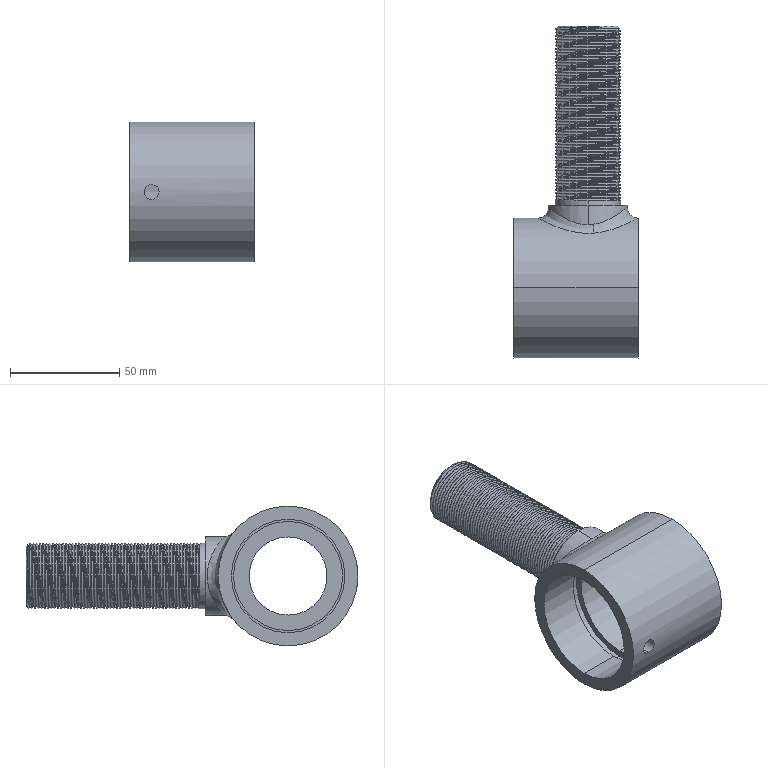Part | SolidWorks | features ICE 2, Chamfer 1, Fillet 1, Helix 1, HoleWzd 1, Revolution 1, SweepCut 1 | 1 solid | 135 faces | box 57 x 152 x 64 mm | volume 133445 mm3 | cylinder 118 | plane 8 | cone 5 | spline 4 | commonest cylinder face diameters 30 x106 6.8 x2 36 x2 50 x2 52 x2 56 x2